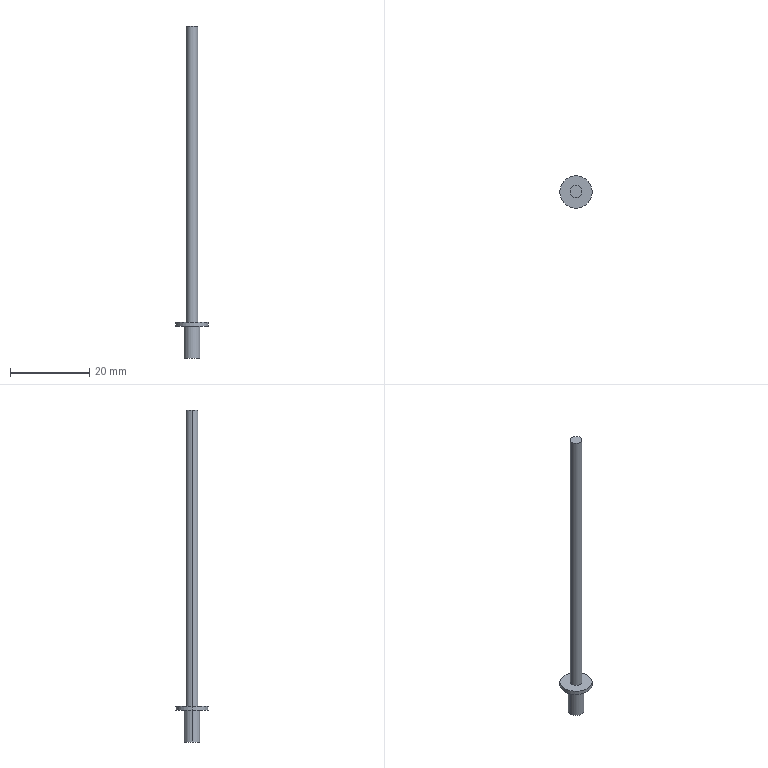Part | Creo | 1 solid | 10 faces | box 8.2 x 8.2 x 84 mm | volume 683.485 mm3 | cylinder 6 | plane 4 | commonest cylinder face diameters 3 x2 4 x2 8.2 x2
STEP:
#1=CARTESIAN_POINT('',(0.,0.,0.));
#2=DIRECTION('',(0.,0.,1.));
#3=DIRECTION('',(1.,0.,0.));
#4=AXIS2_PLACEMENT_3D('',#1,#2,#3);
#5=CARTESIAN_POINT('',(-40.,-81.,-54.09));
#6=VERTEX_POINT('',#5);
#7=CARTESIAN_POINT('',(-37.,-81.,-54.09));
#8=VERTEX_POINT('',#7);
#9=CARTESIAN_POINT('',(-38.5,-81.,-54.09));
#10=DIRECTION('',(0.,0.,-1.));
#11=DIRECTION('',(-1.,0.,0.));
#12=AXIS2_PLACEMENT_3D('',#9,#10,#11);
#13=CIRCLE('',#12,1.5);
#14=EDGE_CURVE('',#6,#8,#13,.T.);
#15=ORIENTED_EDGE('',*,*,#14,.T.);
#16=CARTESIAN_POINT('',(-37.,-81.,20.91));
#17=VERTEX_POINT('',#16);
#18=CARTESIAN_POINT('',(-37.,-81.,20.91));
#19=DIRECTION('',(0.,0.,-1.));
#20=VECTOR('',#19,75.);
#21=LINE('',#18,#20);
#22=EDGE_CURVE('',#17,#8,#21,.T.);
#23=ORIENTED_EDGE('',*,*,#22,.F.);
#24=CARTESIAN_POINT('',(-40.,-81.,20.91));
#25=VERTEX_POINT('',#24);
#26=CARTESIAN_POINT('',(-38.5,-81.,20.91));
#27=DIRECTION('',(0.,0.,1.));
#28=DIRECTION('',(1.,0.,0.));
#29=AXIS2_PLACEMENT_3D('',#26,#27,#28);
#30=CIRCLE('',#29,1.5);
#31=EDGE_CURVE('',#17,#25,#30,.T.);
#32=ORIENTED_EDGE('',*,*,#31,.T.);
#33=CARTESIAN_POINT('',(-40.,-81.,20.91));
#34=DIRECTION('',(0.,0.,-1.));
#35=VECTOR('',#34,75.);
#36=LINE('',#33,#35);
#37=EDGE_CURVE('',#25,#6,#36,.T.);
#38=ORIENTED_EDGE('',*,*,#37,.T.);
#39=EDGE_LOOP('',(#15,#23,#32,#38));
#40=FACE_OUTER_BOUND('',#39,.F.);
#41=CARTESIAN_POINT('',(-38.5,-81.,20.91));
#42=DIRECTION('',(0.,0.,-1.));
#43=DIRECTION('',(-1.,0.,0.));
#44=AXIS2_PLACEMENT_3D('',#41,#42,#43);
#45=CYLINDRICAL_SURFACE('',#44,1.5);
#46=ADVANCED_FACE('',(#40),#45,.T.);
#47=CARTESIAN_POINT('',(-42.6,-81.,-54.09));
#48=VERTEX_POINT('',#47);
#49=CARTESIAN_POINT('',(-34.4,-81.,-54.09));
#50=VERTEX_POINT('',#49);
#51=CARTESIAN_POINT('',(-38.5,-81.,-54.09));
#52=DIRECTION('',(0.,0.,1.));
#53=DIRECTION('',(-1.,0.,0.));
#54=AXIS2_PLACEMENT_3D('',#51,#52,#53);
#55=CIRCLE('',#54,4.1);
#56=EDGE_CURVE('',#48,#50,#55,.T.);
#57=ORIENTED_EDGE('',*,*,#56,.F.);
#58=CARTESIAN_POINT('',(-38.5,-81.,-54.09));
#59=DIRECTION('',(0.,0.,1.));
#60=DIRECTION('',(1.,0.,0.));
#61=AXIS2_PLACEMENT_3D('',#58,#59,#60);
#62=CIRCLE('',#61,4.1);
#63=EDGE_CURVE('',#50,#48,#62,.T.);
#64=ORIENTED_EDGE('',*,*,#63,.F.);
#65=EDGE_LOOP('',(#57,#64));
#66=FACE_OUTER_BOUND('',#65,.F.);
#67=ORIENTED_EDGE('',*,*,#14,.F.);
#68=CARTESIAN_POINT('',(-38.5,-81.,-54.09));
#69=DIRECTION('',(0.,0.,-1.));
#70=DIRECTION('',(1.,0.,0.));
#71=AXIS2_PLACEMENT_3D('',#68,#69,#70);
#72=CIRCLE('',#71,1.5);
#73=EDGE_CURVE('',#8,#6,#72,.T.);
#74=ORIENTED_EDGE('',*,*,#73,.F.);
#75=EDGE_LOOP('',(#67,#74));
#76=FACE_BOUND('',#75,.F.);
#77=CARTESIAN_POINT('',(0.,0.,-54.09));
#78=DIRECTION('',(0.,0.,-1.));
#79=DIRECTION('',(-1.,0.,0.));
#80=AXIS2_PLACEMENT_3D('',#77,#78,#79);
#81=PLANE('',#80);
#82=ADVANCED_FACE('',(#66,#76),#81,.F.);
#83=ORIENTED_EDGE('',*,*,#73,.T.);
#84=ORIENTED_EDGE('',*,*,#37,.F.);
#85=CARTESIAN_POINT('',(-38.5,-81.,20.91));
#86=DIRECTION('',(0.,0.,1.));
#87=DIRECTION('',(-1.,0.,0.));
#88=AXIS2_PLACEMENT_3D('',#85,#86,#87);
#89=CIRCLE('',#88,1.5);
#90=EDGE_CURVE('',#25,#17,#89,.T.);
#91=ORIENTED_EDGE('',*,*,#90,.T.);
#92=ORIENTED_EDGE('',*,*,#22,.T.);
#93=EDGE_LOOP('',(#83,#84,#91,#92));
#94=FACE_OUTER_BOUND('',#93,.F.);
#95=CARTESIAN_POINT('',(-38.5,-81.,20.91));
#96=DIRECTION('',(0.,0.,-1.));
#97=DIRECTION('',(-1.,0.,0.));
#98=AXIS2_PLACEMENT_3D('',#95,#96,#97);
#99=CYLINDRICAL_SURFACE('',#98,1.5);
#100=ADVANCED_FACE('',(#94),#99,.T.);
#101=ORIENTED_EDGE('',*,*,#90,.F.);
#102=ORIENTED_EDGE('',*,*,#31,.F.);
#103=EDGE_LOOP('',(#101,#102));
#104=FACE_OUTER_BOUND('',#103,.F.);
#105=CARTESIAN_POINT('',(-38.5,-81.,20.91));
#106=DIRECTION('',(0.,0.,-1.));
#107=DIRECTION('',(-1.,0.,0.));
#108=AXIS2_PLACEMENT_3D('',#105,#106,#107);
#109=PLANE('',#108);
#110=ADVANCED_FACE('',(#104),#109,.F.);
#111=ORIENTED_EDGE('',*,*,#56,.T.);
#112=CARTESIAN_POINT('',(-34.4,-81.,-55.09));
#113=VERTEX_POINT('',#112);
#114=CARTESIAN_POINT('',(-34.4,-81.,-55.09));
#115=DIRECTION('',(0.,0.,1.));
#116=VECTOR('',#115,1.);
#117=LINE('',#114,#116);
#118=EDGE_CURVE('',#113,#50,#117,.T.);
#119=ORIENTED_EDGE('',*,*,#118,.F.);
#120=CARTESIAN_POINT('',(-42.6,-81.,-55.09));
#121=VERTEX_POINT('',#120);
#122=CARTESIAN_POINT('',(-38.5,-81.,-55.09));
#123=DIRECTION('',(0.,0.,-1.));
#124=DIRECTION('',(1.,0.,0.));
#125=AXIS2_PLACEMENT_3D('',#122,#123,#124);
#126=CIRCLE('',#125,4.1);
#127=EDGE_CURVE('',#113,#121,#126,.T.);
#128=ORIENTED_EDGE('',*,*,#127,.T.);
#129=CARTESIAN_POINT('',(-42.6,-81.,-55.09));
#130=DIRECTION('',(0.,0.,1.));
#131=VECTOR('',#130,1.);
#132=LINE('',#129,#131);
#133=EDGE_CURVE('',#121,#48,#132,.T.);
#134=ORIENTED_EDGE('',*,*,#133,.T.);
#135=EDGE_LOOP('',(#111,#119,#128,#134));
#136=FACE_OUTER_BOUND('',#135,.F.);
#137=CARTESIAN_POINT('',(-38.5,-81.,-90.09));
#138=DIRECTION('',(0.,0.,1.));
#139=DIRECTION('',(1.,0.,0.));
#140=AXIS2_PLACEMENT_3D('',#137,#138,#139);
#141=CYLINDRICAL_SURFACE('',#140,4.1);
#142=ADVANCED_FACE('',(#136),#141,.T.);
#143=ORIENTED_EDGE('',*,*,#63,.T.);
#144=ORIENTED_EDGE('',*,*,#133,.F.);
#145=CARTESIAN_POINT('',(-38.5,-81.,-55.09));
#146=DIRECTION('',(0.,0.,-1.));
#147=DIRECTION('',(-1.,0.,0.));
#148=AXIS2_PLACEMENT_3D('',#145,#146,#147);
#149=CIRCLE('',#148,4.1);
#150=EDGE_CURVE('',#121,#113,#149,.T.);
#151=ORIENTED_EDGE('',*,*,#150,.T.);
#152=ORIENTED_EDGE('',*,*,#118,.T.);
#153=EDGE_LOOP('',(#143,#144,#151,#152));
#154=FACE_OUTER_BOUND('',#153,.F.);
#155=CARTESIAN_POINT('',(-38.5,-81.,-90.09));
#156=DIRECTION('',(0.,0.,1.));
#157=DIRECTION('',(1.,0.,0.));
#158=AXIS2_PLACEMENT_3D('',#155,#156,#157);
#159=CYLINDRICAL_SURFACE('',#158,4.1);
#160=ADVANCED_FACE('',(#154),#159,.T.);
#161=ORIENTED_EDGE('',*,*,#150,.F.);
#162=ORIENTED_EDGE('',*,*,#127,.F.);
#163=EDGE_LOOP('',(#161,#162));
#164=FACE_OUTER_BOUND('',#163,.F.);
#165=CARTESIAN_POINT('',(-36.5,-81.,-55.09));
#166=VERTEX_POINT('',#165);
#167=CARTESIAN_POINT('',(-40.5,-81.,-55.09));
#168=VERTEX_POINT('',#167);
#169=CARTESIAN_POINT('',(-38.5,-81.,-55.09));
#170=DIRECTION('',(0.,0.,1.));
#171=DIRECTION('',(1.,0.,0.));
#172=AXIS2_PLACEMENT_3D('',#169,#170,#171);
#173=CIRCLE('',#172,2.);
#174=EDGE_CURVE('',#166,#168,#173,.T.);
#175=ORIENTED_EDGE('',*,*,#174,.F.);
#176=CARTESIAN_POINT('',(-38.5,-81.,-55.09));
#177=DIRECTION('',(0.,0.,1.));
#178=DIRECTION('',(-1.,0.,0.));
#179=AXIS2_PLACEMENT_3D('',#176,#177,#178);
#180=CIRCLE('',#179,2.);
#181=EDGE_CURVE('',#168,#166,#180,.T.);
#182=ORIENTED_EDGE('',*,*,#181,.F.);
#183=EDGE_LOOP('',(#175,#182));
#184=FACE_BOUND('',#183,.F.);
#185=CARTESIAN_POINT('',(0.,0.,-55.09));
#186=DIRECTION('',(0.,0.,-1.));
#187=DIRECTION('',(-1.,0.,0.));
#188=AXIS2_PLACEMENT_3D('',#185,#186,#187);
#189=PLANE('',#188);
#190=ADVANCED_FACE('',(#164,#184),#189,.T.);
#191=CARTESIAN_POINT('',(-40.5,-81.,-63.09));
#192=VERTEX_POINT('',#191);
#193=CARTESIAN_POINT('',(-36.5,-81.,-63.09));
#194=VERTEX_POINT('',#193);
#195=CARTESIAN_POINT('',(-38.5,-81.,-63.09));
#196=DIRECTION('',(0.,0.,-1.));
#197=DIRECTION('',(-1.,0.,0.));
#198=AXIS2_PLACEMENT_3D('',#195,#196,#197);
#199=CIRCLE('',#198,2.);
#200=EDGE_CURVE('',#192,#194,#199,.T.);
#201=ORIENTED_EDGE('',*,*,#200,.T.);
#202=CARTESIAN_POINT('',(-36.5,-81.,-63.09));
#203=DIRECTION('',(0.,0.,1.));
#204=VECTOR('',#203,8.);
#205=LINE('',#202,#204);
#206=EDGE_CURVE('',#194,#166,#205,.T.);
#207=ORIENTED_EDGE('',*,*,#206,.T.);
#208=ORIENTED_EDGE('',*,*,#174,.T.);
#209=CARTESIAN_POINT('',(-40.5,-81.,-63.09));
#210=DIRECTION('',(0.,0.,1.));
#211=VECTOR('',#210,8.);
#212=LINE('',#209,#211);
#213=EDGE_CURVE('',#192,#168,#212,.T.);
#214=ORIENTED_EDGE('',*,*,#213,.F.);
#215=EDGE_LOOP('',(#201,#207,#208,#214));
#216=FACE_OUTER_BOUND('',#215,.F.);
#217=CARTESIAN_POINT('',(-38.5,-81.,-90.09));
#218=DIRECTION('',(0.,0.,1.));
#219=DIRECTION('',(1.,0.,0.));
#220=AXIS2_PLACEMENT_3D('',#217,#218,#219);
#221=CYLINDRICAL_SURFACE('',#220,2.);
#222=ADVANCED_FACE('',(#216),#221,.T.);
#223=CARTESIAN_POINT('',(-38.5,-81.,-63.09));
#224=DIRECTION('',(0.,0.,-1.));
#225=DIRECTION('',(1.,0.,0.));
#226=AXIS2_PLACEMENT_3D('',#223,#224,#225);
#227=CIRCLE('',#226,2.);
#228=EDGE_CURVE('',#194,#192,#227,.T.);
#229=ORIENTED_EDGE('',*,*,#228,.F.);
#230=ORIENTED_EDGE('',*,*,#200,.F.);
#231=EDGE_LOOP('',(#229,#230));
#232=FACE_OUTER_BOUND('',#231,.F.);
#233=CARTESIAN_POINT('',(-38.5,-81.,-63.09));
#234=DIRECTION('',(0.,0.,1.));
#235=DIRECTION('',(1.,0.,0.));
#236=AXIS2_PLACEMENT_3D('',#233,#234,#235);
#237=PLANE('',#236);
#238=ADVANCED_FACE('',(#232),#237,.F.);
#239=ORIENTED_EDGE('',*,*,#228,.T.);
#240=ORIENTED_EDGE('',*,*,#213,.T.);
#241=ORIENTED_EDGE('',*,*,#181,.T.);
#242=ORIENTED_EDGE('',*,*,#206,.F.);
#243=EDGE_LOOP('',(#239,#240,#241,#242));
#244=FACE_OUTER_BOUND('',#243,.F.);
#245=CARTESIAN_POINT('',(-38.5,-81.,-90.09));
#246=DIRECTION('',(0.,0.,1.));
#247=DIRECTION('',(1.,0.,0.));
#248=AXIS2_PLACEMENT_3D('',#245,#246,#247);
#249=CYLINDRICAL_SURFACE('',#248,2.);
#250=ADVANCED_FACE('',(#244),#249,.T.);
#251=CLOSED_SHELL('',(#46,#82,#100,#110,#142,#160,#190,#222,#238,#250));
#252=MANIFOLD_SOLID_BREP('',#251);
#253=(LENGTH_UNIT()NAMED_UNIT(*)SI_UNIT(.MILLI.,.METRE.));
#254=UNCERTAINTY_MEASURE_WITH_UNIT(LENGTH_MEASURE(0.008479),#253,'','');
#255=(NAMED_UNIT(*)PLANE_ANGLE_UNIT()SI_UNIT($,.RADIAN.));
#256=PLANE_ANGLE_MEASURE_WITH_UNIT(PLANE_ANGLE_MEASURE(0.01745),#255);
#257=(CONVERSION_BASED_UNIT('DEGREE',#256)NAMED_UNIT(*)PLANE_ANGLE_UNIT());
#258=(NAMED_UNIT(*)SI_UNIT($,.STERADIAN.)SOLID_ANGLE_UNIT());
#259=(GEOMETRIC_REPRESENTATION_CONTEXT(3)GLOBAL_UNCERTAINTY_ASSIGNED_CONTEXT((#254))GLOBAL_UNIT_ASSIGNED_CONTEXT((#253,#257,#258))REPRESENTATION_CONTEXT('',''));
#260=ADVANCED_BREP_SHAPE_REPRESENTATION('',(#4,#252),#259);